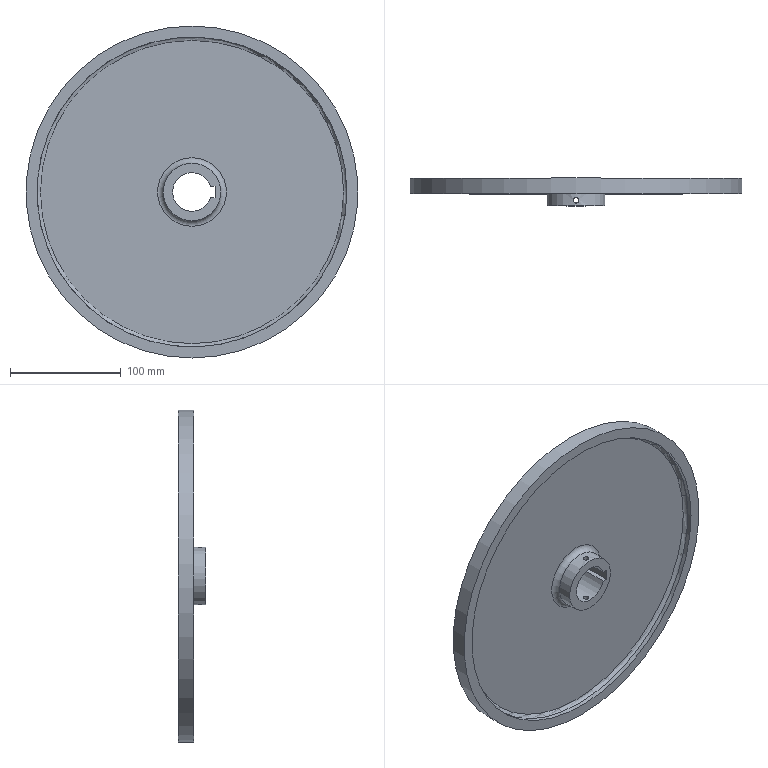Part | NX | features DATUM_CSYS 5, SKETCH 4, EXTRUDE 3, BLEND 2, DATUM_PLANE 1, SWP104 1 | 1 solid | 15 faces | box 300 x 25 x 300 mm | volume 574128 mm3 | plane 7 | cylinder 6 | torus 2 | commonest cylinder face diameters 5 x2 35 x1 52 x1 280 x1 300 x1
STEP:
#1=CARTESIAN_POINT('',(16.771,0.,5.));
#2=VERTEX_POINT('',#1);
#3=CARTESIAN_POINT('',(16.771,0.,-5.));
#4=VERTEX_POINT('',#3);
#5=CARTESIAN_POINT('',(0.,0.,0.));
#6=DIRECTION('',(0.,-1.,0.));
#7=DIRECTION('',(0.,0.,-1.));
#8=AXIS2_PLACEMENT_3D('',#5,#6,#7);
#9=CIRCLE('',#8,17.5);
#10=EDGE_CURVE('',#2,#4,#9,.T.);
#11=ORIENTED_EDGE('',*,*,#10,.T.);
#12=CARTESIAN_POINT('',(16.771,25.,-5.));
#13=VERTEX_POINT('',#12);
#14=CARTESIAN_POINT('',(16.771,0.,-5.));
#15=DIRECTION('',(0.,-1.,0.));
#16=VECTOR('',#15,1000.);
#17=LINE('',#14,#16);
#18=EDGE_CURVE('',#4,#13,#17,.F.);
#19=ORIENTED_EDGE('',*,*,#18,.T.);
#20=CARTESIAN_POINT('',(16.771,25.,5.));
#21=VERTEX_POINT('',#20);
#22=CARTESIAN_POINT('',(0.,25.,0.));
#23=DIRECTION('',(0.,-1.,0.));
#24=DIRECTION('',(0.,0.,-1.));
#25=AXIS2_PLACEMENT_3D('',#22,#23,#24);
#26=CIRCLE('',#25,17.5);
#27=EDGE_CURVE('',#21,#13,#26,.T.);
#28=ORIENTED_EDGE('',*,*,#27,.F.);
#29=CARTESIAN_POINT('',(16.771,0.,5.));
#30=DIRECTION('',(0.,-1.,0.));
#31=VECTOR('',#30,1000.);
#32=LINE('',#29,#31);
#33=EDGE_CURVE('',#21,#2,#32,.T.);
#34=ORIENTED_EDGE('',*,*,#33,.T.);
#35=EDGE_LOOP('',(#11,#19,#28,#34));
#36=FACE_BOUND('',#35,.T.);
#37=CARTESIAN_POINT('',(2.5,5.,17.321));
#38=VERTEX_POINT('',#37);
#39=CARTESIAN_POINT('',(1.957,6.961,17.411));
#40=CARTESIAN_POINT('',(2.771,5.,17.275));
#41=CARTESIAN_POINT('',(1.958,3.041,17.411));
#42=CARTESIAN_POINT('',(0.002312,2.23,17.545));
#43=CARTESIAN_POINT('',(-1.959,3.04,17.411));
#44=CARTESIAN_POINT('',(-2.77,4.999,17.275));
#45=CARTESIAN_POINT('',(-1.961,6.957,17.41));
#46=CARTESIAN_POINT('',(-0.002322,7.771,17.545));
#47=CARTESIAN_POINT('',(1.957,6.961,17.411));
#48=CARTESIAN_POINT('',(2.771,5.,17.275));
#49=CARTESIAN_POINT('',(1.958,3.041,17.411));
#50=B_SPLINE_CURVE_WITH_KNOTS('',3,(#39,#40,#41,#42,#43,#44,#45,#46,#47,#48,#49),.UNSPECIFIED.,.T.,.F.,(1,1,1,1,1,1,1,1,1,1,1,1,1,1,1),(-0.005869,-0.003913,-0.001956,0.,0.001956,0.003913,0.005869,0.007825,0.009781,0.01174,0.01369,0.01565,0.01761,0.01956,0.02152),.UNSPECIFIED.);
#51=EDGE_CURVE('',#38,#38,#50,.T.);
#52=ORIENTED_EDGE('',*,*,#51,.F.);
#53=EDGE_LOOP('',(#52));
#54=FACE_BOUND('',#53,.T.);
#55=CARTESIAN_POINT('',(2.5,5.,-17.321));
#56=VERTEX_POINT('',#55);
#57=CARTESIAN_POINT('',(1.957,3.039,-17.411));
#58=CARTESIAN_POINT('',(2.771,5.,-17.275));
#59=CARTESIAN_POINT('',(1.958,6.959,-17.411));
#60=CARTESIAN_POINT('',(0.002312,7.77,-17.545));
#61=CARTESIAN_POINT('',(-1.959,6.96,-17.411));
#62=CARTESIAN_POINT('',(-2.77,5.001,-17.275));
#63=CARTESIAN_POINT('',(-1.961,3.043,-17.41));
#64=CARTESIAN_POINT('',(-0.002322,2.229,-17.545));
#65=CARTESIAN_POINT('',(1.957,3.039,-17.411));
#66=CARTESIAN_POINT('',(2.771,5.,-17.275));
#67=CARTESIAN_POINT('',(1.958,6.959,-17.411));
#68=B_SPLINE_CURVE_WITH_KNOTS('',3,(#57,#58,#59,#60,#61,#62,#63,#64,#65,#66,#67),.UNSPECIFIED.,.T.,.F.,(1,1,1,1,1,1,1,1,1,1,1,1,1,1,1),(-0.005869,-0.003913,-0.001956,0.,0.001956,0.003913,0.005869,0.007825,0.009781,0.01174,0.01369,0.01565,0.01761,0.01956,0.02152),.UNSPECIFIED.);
#69=EDGE_CURVE('',#56,#56,#68,.T.);
#70=ORIENTED_EDGE('',*,*,#69,.F.);
#71=EDGE_LOOP('',(#70));
#72=FACE_BOUND('',#71,.T.);
#73=CARTESIAN_POINT('',(0.,0.,0.));
#74=DIRECTION('',(0.,-1.,0.));
#75=DIRECTION('',(0.,0.,-1.));
#76=AXIS2_PLACEMENT_3D('',#73,#74,#75);
#77=CYLINDRICAL_SURFACE('',#76,17.5);
#78=ADVANCED_FACE('',(#36,#54,#72),#77,.F.);
#79=CARTESIAN_POINT('',(0.,13.,-26.));
#80=VERTEX_POINT('',#79);
#81=CARTESIAN_POINT('',(0.,13.,0.));
#82=DIRECTION('',(0.,-1.,0.));
#83=DIRECTION('',(0.,0.,-1.));
#84=AXIS2_PLACEMENT_3D('',#81,#82,#83);
#85=CIRCLE('',#84,26.);
#86=EDGE_CURVE('',#80,#80,#85,.T.);
#87=ORIENTED_EDGE('',*,*,#86,.T.);
#88=EDGE_LOOP('',(#87));
#89=FACE_BOUND('',#88,.T.);
#90=CARTESIAN_POINT('',(0.,0.,-26.));
#91=VERTEX_POINT('',#90);
#92=CARTESIAN_POINT('',(0.,0.,0.));
#93=DIRECTION('',(0.,-1.,0.));
#94=DIRECTION('',(0.,0.,-1.));
#95=AXIS2_PLACEMENT_3D('',#92,#93,#94);
#96=CIRCLE('',#95,26.);
#97=EDGE_CURVE('',#91,#91,#96,.T.);
#98=ORIENTED_EDGE('',*,*,#97,.F.);
#99=EDGE_LOOP('',(#98));
#100=FACE_BOUND('',#99,.T.);
#101=CARTESIAN_POINT('',(2.5,5.,25.88));
#102=VERTEX_POINT('',#101);
#103=CARTESIAN_POINT('',(1.957,3.039,25.94));
#104=CARTESIAN_POINT('',(2.771,5.,25.849));
#105=CARTESIAN_POINT('',(1.958,6.959,25.94));
#106=CARTESIAN_POINT('',(0.002151,7.77,26.03));
#107=CARTESIAN_POINT('',(-1.958,6.96,25.94));
#108=CARTESIAN_POINT('',(-2.77,5.,25.849));
#109=CARTESIAN_POINT('',(-1.961,3.043,25.94));
#110=CARTESIAN_POINT('',(-0.002705,2.229,26.03));
#111=CARTESIAN_POINT('',(1.957,3.039,25.94));
#112=CARTESIAN_POINT('',(2.771,5.,25.849));
#113=CARTESIAN_POINT('',(1.958,6.959,25.94));
#114=B_SPLINE_CURVE_WITH_KNOTS('',3,(#103,#104,#105,#106,#107,#108,#109,#110,#111,#112,#113),.UNSPECIFIED.,.T.,.F.,(1,1,1,1,1,1,1,1,1,1,1,1,1,1,1),(-0.005865,-0.00391,-0.001955,0.,0.001955,0.00391,0.005865,0.00782,0.009775,0.01173,0.01368,0.01564,0.01759,0.01955,0.0215),.UNSPECIFIED.);
#115=EDGE_CURVE('',#102,#102,#114,.T.);
#116=ORIENTED_EDGE('',*,*,#115,.F.);
#117=EDGE_LOOP('',(#116));
#118=FACE_BOUND('',#117,.T.);
#119=CARTESIAN_POINT('',(0.,7.5,-26.));
#120=VERTEX_POINT('',#119);
#121=CARTESIAN_POINT('',(-1.961,6.957,-25.94));
#122=CARTESIAN_POINT('',(0.0004919,7.771,-26.03));
#123=CARTESIAN_POINT('',(1.959,6.958,-25.94));
#124=CARTESIAN_POINT('',(2.77,5.002,-25.849));
#125=CARTESIAN_POINT('',(1.96,3.042,-25.94));
#126=CARTESIAN_POINT('',(0.0004793,2.23,-26.03));
#127=CARTESIAN_POINT('',(-1.957,3.039,-25.94));
#128=CARTESIAN_POINT('',(-2.771,4.997,-25.849));
#129=CARTESIAN_POINT('',(-1.961,6.957,-25.94));
#130=CARTESIAN_POINT('',(0.0004919,7.771,-26.03));
#131=CARTESIAN_POINT('',(1.959,6.958,-25.94));
#132=B_SPLINE_CURVE_WITH_KNOTS('',3,(#121,#122,#123,#124,#125,#126,#127,#128,#129,#130,#131),.UNSPECIFIED.,.T.,.F.,(1,1,1,1,1,1,1,1,1,1,1,1,1,1,1),(-0.005865,-0.00391,-0.001955,0.,0.001955,0.00391,0.005865,0.00782,0.009775,0.01173,0.01368,0.01564,0.01759,0.01955,0.0215),.UNSPECIFIED.);
#133=EDGE_CURVE('',#120,#120,#132,.T.);
#134=ORIENTED_EDGE('',*,*,#133,.F.);
#135=EDGE_LOOP('',(#134));
#136=FACE_BOUND('',#135,.T.);
#137=CARTESIAN_POINT('',(0.,0.,0.));
#138=DIRECTION('',(0.,-1.,0.));
#139=DIRECTION('',(0.,0.,-1.));
#140=AXIS2_PLACEMENT_3D('',#137,#138,#139);
#141=CYLINDRICAL_SURFACE('',#140,26.);
#142=ADVANCED_FACE('',(#89,#100,#118,#136),#141,.T.);
#143=CARTESIAN_POINT('',(20.828,0.,5.));
#144=VERTEX_POINT('',#143);
#145=CARTESIAN_POINT('',(20.828,0.,-5.));
#146=VERTEX_POINT('',#145);
#147=CARTESIAN_POINT('',(20.828,0.,26.));
#148=DIRECTION('',(0.,0.,-1.));
#149=VECTOR('',#148,1000.);
#150=LINE('',#147,#149);
#151=EDGE_CURVE('',#144,#146,#150,.T.);
#152=ORIENTED_EDGE('',*,*,#151,.T.);
#153=CARTESIAN_POINT('',(0.,0.,-5.));
#154=DIRECTION('',(-1.,0.,0.));
#155=VECTOR('',#154,1000.);
#156=LINE('',#153,#155);
#157=EDGE_CURVE('',#146,#4,#156,.T.);
#158=ORIENTED_EDGE('',*,*,#157,.T.);
#159=ORIENTED_EDGE('',*,*,#10,.F.);
#160=CARTESIAN_POINT('',(0.,0.,5.));
#161=DIRECTION('',(1.,0.,0.));
#162=VECTOR('',#161,1000.);
#163=LINE('',#160,#162);
#164=EDGE_CURVE('',#2,#144,#163,.T.);
#165=ORIENTED_EDGE('',*,*,#164,.T.);
#166=EDGE_LOOP('',(#152,#158,#159,#165));
#167=FACE_BOUND('',#166,.T.);
#168=ORIENTED_EDGE('',*,*,#97,.T.);
#169=EDGE_LOOP('',(#168));
#170=FACE_BOUND('',#169,.T.);
#171=CARTESIAN_POINT('',(0.,0.,26.));
#172=DIRECTION('',(0.,1.,0.));
#173=DIRECTION('',(0.,0.,1.));
#174=AXIS2_PLACEMENT_3D('',#171,#172,#173);
#175=PLANE('',#174);
#176=ADVANCED_FACE('',(#167,#170),#175,.F.);
#177=CARTESIAN_POINT('',(0.,25.,-150.));
#178=VERTEX_POINT('',#177);
#179=CARTESIAN_POINT('',(0.,25.,0.));
#180=DIRECTION('',(0.,-1.,0.));
#181=DIRECTION('',(0.,0.,-1.));
#182=AXIS2_PLACEMENT_3D('',#179,#180,#181);
#183=CIRCLE('',#182,150.);
#184=EDGE_CURVE('',#178,#178,#183,.T.);
#185=ORIENTED_EDGE('',*,*,#184,.F.);
#186=EDGE_LOOP('',(#185));
#187=FACE_BOUND('',#186,.T.);
#188=ORIENTED_EDGE('',*,*,#27,.T.);
#189=CARTESIAN_POINT('',(20.828,25.,-5.));
#190=VERTEX_POINT('',#189);
#191=CARTESIAN_POINT('',(0.,25.,-5.));
#192=DIRECTION('',(1.,0.,0.));
#193=VECTOR('',#192,1000.);
#194=LINE('',#191,#193);
#195=EDGE_CURVE('',#13,#190,#194,.T.);
#196=ORIENTED_EDGE('',*,*,#195,.T.);
#197=CARTESIAN_POINT('',(20.828,25.,5.));
#198=VERTEX_POINT('',#197);
#199=CARTESIAN_POINT('',(20.828,25.,17.5));
#200=DIRECTION('',(0.,0.,1.));
#201=VECTOR('',#200,1000.);
#202=LINE('',#199,#201);
#203=EDGE_CURVE('',#190,#198,#202,.T.);
#204=ORIENTED_EDGE('',*,*,#203,.T.);
#205=CARTESIAN_POINT('',(0.,25.,5.));
#206=DIRECTION('',(-1.,0.,0.));
#207=VECTOR('',#206,1000.);
#208=LINE('',#205,#207);
#209=EDGE_CURVE('',#198,#21,#208,.T.);
#210=ORIENTED_EDGE('',*,*,#209,.T.);
#211=EDGE_LOOP('',(#188,#196,#204,#210));
#212=FACE_BOUND('',#211,.T.);
#213=CARTESIAN_POINT('',(0.,25.,17.5));
#214=DIRECTION('',(0.,-1.,0.));
#215=DIRECTION('',(0.,0.,-1.));
#216=AXIS2_PLACEMENT_3D('',#213,#214,#215);
#217=PLANE('',#216);
#218=ADVANCED_FACE('',(#187,#212),#217,.F.);
#219=CARTESIAN_POINT('',(0.,11.,-150.));
#220=VERTEX_POINT('',#219);
#221=CARTESIAN_POINT('',(0.,11.,0.));
#222=DIRECTION('',(0.,-1.,0.));
#223=DIRECTION('',(0.,0.,-1.));
#224=AXIS2_PLACEMENT_3D('',#221,#222,#223);
#225=CIRCLE('',#224,150.);
#226=EDGE_CURVE('',#220,#220,#225,.T.);
#227=ORIENTED_EDGE('',*,*,#226,.F.);
#228=EDGE_LOOP('',(#227));
#229=FACE_BOUND('',#228,.T.);
#230=ORIENTED_EDGE('',*,*,#184,.T.);
#231=EDGE_LOOP('',(#230));
#232=FACE_BOUND('',#231,.T.);
#233=CARTESIAN_POINT('',(0.,0.,0.));
#234=DIRECTION('',(0.,-1.,0.));
#235=DIRECTION('',(0.,0.,-1.));
#236=AXIS2_PLACEMENT_3D('',#233,#234,#235);
#237=CYLINDRICAL_SURFACE('',#236,150.);
#238=ADVANCED_FACE('',(#229,#232),#237,.T.);
#239=CARTESIAN_POINT('',(140.,11.,0.));
#240=VERTEX_POINT('',#239);
#241=CARTESIAN_POINT('',(0.,11.,0.));
#242=DIRECTION('',(0.,-1.,0.));
#243=DIRECTION('',(1.,0.,0.));
#244=AXIS2_PLACEMENT_3D('',#241,#242,#243);
#245=CIRCLE('',#244,140.);
#246=EDGE_CURVE('',#240,#240,#245,.T.);
#247=ORIENTED_EDGE('',*,*,#246,.F.);
#248=EDGE_LOOP('',(#247));
#249=FACE_BOUND('',#248,.T.);
#250=ORIENTED_EDGE('',*,*,#226,.T.);
#251=EDGE_LOOP('',(#250));
#252=FACE_BOUND('',#251,.T.);
#253=CARTESIAN_POINT('',(0.,11.,150.));
#254=DIRECTION('',(0.,1.,0.));
#255=DIRECTION('',(0.,0.,1.));
#256=AXIS2_PLACEMENT_3D('',#253,#254,#255);
#257=PLANE('',#256);
#258=ADVANCED_FACE('',(#249,#252),#257,.F.);
#259=CARTESIAN_POINT('',(0.,15.,-140.));
#260=VERTEX_POINT('',#259);
#261=CARTESIAN_POINT('',(0.,15.,0.));
#262=DIRECTION('',(0.,-1.,0.));
#263=DIRECTION('',(0.,0.,-1.));
#264=AXIS2_PLACEMENT_3D('',#261,#262,#263);
#265=CIRCLE('',#264,140.);
#266=EDGE_CURVE('',#260,#260,#265,.F.);
#267=ORIENTED_EDGE('',*,*,#266,.T.);
#268=EDGE_LOOP('',(#267));
#269=FACE_BOUND('',#268,.T.);
#270=ORIENTED_EDGE('',*,*,#246,.T.);
#271=EDGE_LOOP('',(#270));
#272=FACE_BOUND('',#271,.T.);
#273=CARTESIAN_POINT('',(0.,11.,0.));
#274=DIRECTION('',(0.,1.,0.));
#275=DIRECTION('',(0.,0.,1.));
#276=AXIS2_PLACEMENT_3D('',#273,#274,#275);
#277=CYLINDRICAL_SURFACE('',#276,140.);
#278=ADVANCED_FACE('',(#269,#272),#277,.F.);
#279=CARTESIAN_POINT('',(0.,18.,-31.));
#280=VERTEX_POINT('',#279);
#281=CARTESIAN_POINT('',(0.,18.,0.));
#282=DIRECTION('',(0.,-1.,0.));
#283=DIRECTION('',(0.,0.,-1.));
#284=AXIS2_PLACEMENT_3D('',#281,#282,#283);
#285=CIRCLE('',#284,31.);
#286=EDGE_CURVE('',#280,#280,#285,.F.);
#287=ORIENTED_EDGE('',*,*,#286,.T.);
#288=EDGE_LOOP('',(#287));
#289=FACE_BOUND('',#288,.T.);
#290=CARTESIAN_POINT('',(0.,18.,-137.));
#291=VERTEX_POINT('',#290);
#292=CARTESIAN_POINT('',(0.,18.,0.));
#293=DIRECTION('',(0.,-1.,0.));
#294=DIRECTION('',(0.,0.,-1.));
#295=AXIS2_PLACEMENT_3D('',#292,#293,#294);
#296=CIRCLE('',#295,137.);
#297=EDGE_CURVE('',#291,#291,#296,.T.);
#298=ORIENTED_EDGE('',*,*,#297,.T.);
#299=EDGE_LOOP('',(#298));
#300=FACE_BOUND('',#299,.T.);
#301=CARTESIAN_POINT('',(0.,18.,0.));
#302=DIRECTION('',(0.,-1.,0.));
#303=DIRECTION('',(0.,0.,-1.));
#304=AXIS2_PLACEMENT_3D('',#301,#302,#303);
#305=PLANE('',#304);
#306=ADVANCED_FACE('',(#289,#300),#305,.T.);
#307=ORIENTED_EDGE('',*,*,#297,.F.);
#308=EDGE_LOOP('',(#307));
#309=FACE_BOUND('',#308,.T.);
#310=ORIENTED_EDGE('',*,*,#266,.F.);
#311=EDGE_LOOP('',(#310));
#312=FACE_BOUND('',#311,.T.);
#313=CARTESIAN_POINT('',(0.,15.,0.));
#314=DIRECTION('',(0.,-1.,0.));
#315=DIRECTION('',(0.,0.,-1.));
#316=AXIS2_PLACEMENT_3D('',#313,#314,#315);
#317=TOROIDAL_SURFACE('',#316,137.,3.);
#318=ADVANCED_FACE('',(#309,#312),#317,.F.);
#319=ORIENTED_EDGE('',*,*,#286,.F.);
#320=EDGE_LOOP('',(#319));
#321=FACE_BOUND('',#320,.T.);
#322=ORIENTED_EDGE('',*,*,#86,.F.);
#323=EDGE_LOOP('',(#322));
#324=FACE_BOUND('',#323,.T.);
#325=CARTESIAN_POINT('',(0.,13.,0.));
#326=DIRECTION('',(0.,-1.,0.));
#327=DIRECTION('',(0.,0.,-1.));
#328=AXIS2_PLACEMENT_3D('',#325,#326,#327);
#329=TOROIDAL_SURFACE('',#328,31.,5.);
#330=ADVANCED_FACE('',(#321,#324),#329,.F.);
#331=CARTESIAN_POINT('',(20.828,34.,-5.));
#332=DIRECTION('',(0.,-1.,0.));
#333=VECTOR('',#332,1000.);
#334=LINE('',#331,#333);
#335=EDGE_CURVE('',#146,#190,#334,.F.);
#336=ORIENTED_EDGE('',*,*,#335,.T.);
#337=ORIENTED_EDGE('',*,*,#195,.F.);
#338=ORIENTED_EDGE('',*,*,#18,.F.);
#339=ORIENTED_EDGE('',*,*,#157,.F.);
#340=EDGE_LOOP('',(#336,#337,#338,#339));
#341=FACE_BOUND('',#340,.T.);
#342=CARTESIAN_POINT('',(7.828,34.,-5.));
#343=DIRECTION('',(0.,0.,-1.));
#344=DIRECTION('',(-1.,0.,0.));
#345=AXIS2_PLACEMENT_3D('',#342,#343,#344);
#346=PLANE('',#345);
#347=ADVANCED_FACE('',(#341),#346,.F.);
#348=CARTESIAN_POINT('',(20.828,34.,5.));
#349=DIRECTION('',(0.,-1.,0.));
#350=VECTOR('',#349,1000.);
#351=LINE('',#348,#350);
#352=EDGE_CURVE('',#144,#198,#351,.F.);
#353=ORIENTED_EDGE('',*,*,#352,.T.);
#354=ORIENTED_EDGE('',*,*,#203,.F.);
#355=ORIENTED_EDGE('',*,*,#335,.F.);
#356=ORIENTED_EDGE('',*,*,#151,.F.);
#357=EDGE_LOOP('',(#353,#354,#355,#356));
#358=FACE_BOUND('',#357,.T.);
#359=CARTESIAN_POINT('',(20.828,34.,-5.));
#360=DIRECTION('',(1.,0.,0.));
#361=DIRECTION('',(0.,0.,-1.));
#362=AXIS2_PLACEMENT_3D('',#359,#360,#361);
#363=PLANE('',#362);
#364=ADVANCED_FACE('',(#358),#363,.F.);
#365=ORIENTED_EDGE('',*,*,#33,.F.);
#366=ORIENTED_EDGE('',*,*,#209,.F.);
#367=ORIENTED_EDGE('',*,*,#352,.F.);
#368=ORIENTED_EDGE('',*,*,#164,.F.);
#369=EDGE_LOOP('',(#365,#366,#367,#368));
#370=FACE_BOUND('',#369,.T.);
#371=CARTESIAN_POINT('',(20.828,34.,5.));
#372=DIRECTION('',(0.,0.,1.));
#373=DIRECTION('',(1.,0.,0.));
#374=AXIS2_PLACEMENT_3D('',#371,#372,#373);
#375=PLANE('',#374);
#376=ADVANCED_FACE('',(#370),#375,.F.);
#377=ORIENTED_EDGE('',*,*,#115,.T.);
#378=EDGE_LOOP('',(#377));
#379=FACE_BOUND('',#378,.T.);
#380=ORIENTED_EDGE('',*,*,#51,.T.);
#381=EDGE_LOOP('',(#380));
#382=FACE_BOUND('',#381,.T.);
#383=CARTESIAN_POINT('',(0.,5.,-41.));
#384=DIRECTION('',(0.,0.,1.));
#385=DIRECTION('',(1.,0.,0.));
#386=AXIS2_PLACEMENT_3D('',#383,#384,#385);
#387=CYLINDRICAL_SURFACE('',#386,2.5);
#388=ADVANCED_FACE('',(#379,#382),#387,.F.);
#389=ORIENTED_EDGE('',*,*,#133,.T.);
#390=EDGE_LOOP('',(#389));
#391=FACE_BOUND('',#390,.T.);
#392=ORIENTED_EDGE('',*,*,#69,.T.);
#393=EDGE_LOOP('',(#392));
#394=FACE_BOUND('',#393,.T.);
#395=CARTESIAN_POINT('',(0.,5.,-41.));
#396=DIRECTION('',(0.,0.,1.));
#397=DIRECTION('',(1.,0.,0.));
#398=AXIS2_PLACEMENT_3D('',#395,#396,#397);
#399=CYLINDRICAL_SURFACE('',#398,2.5);
#400=ADVANCED_FACE('',(#391,#394),#399,.F.);
#401=CLOSED_SHELL('',(#78,#142,#176,#218,#238,#258,#278,#306,#318,#330,#347,#364,#376,#388,#400));
#402=MANIFOLD_SOLID_BREP('',#401);
#403=(LENGTH_UNIT()NAMED_UNIT(*)SI_UNIT(.MILLI.,.METRE.));
#404=UNCERTAINTY_MEASURE_WITH_UNIT(LENGTH_MEASURE(0.0508),#403,'','');
#405=(NAMED_UNIT(*)PLANE_ANGLE_UNIT()SI_UNIT($,.RADIAN.));
#406=(NAMED_UNIT(*)SI_UNIT($,.STERADIAN.)SOLID_ANGLE_UNIT());
#407=(GEOMETRIC_REPRESENTATION_CONTEXT(3)GLOBAL_UNCERTAINTY_ASSIGNED_CONTEXT((#404))GLOBAL_UNIT_ASSIGNED_CONTEXT((#403,#405,#406))REPRESENTATION_CONTEXT('',''));
#408=ADVANCED_BREP_SHAPE_REPRESENTATION('',(#402),#407);